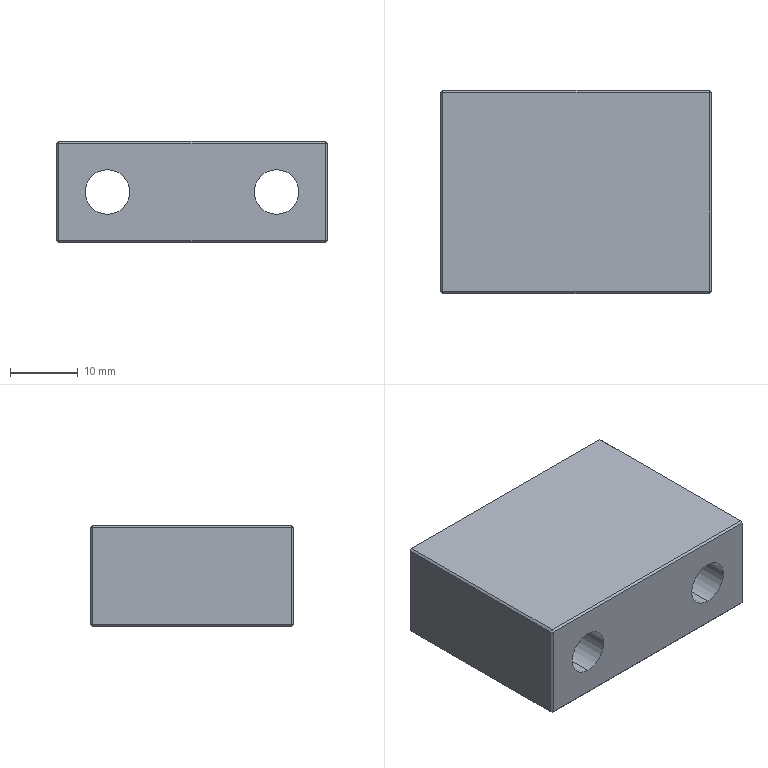Part | SolidWorks | features Chamfer 1, Extrusion 1, HoleWzd 1 | 1 solid | 36 faces | box 40 x 30 x 15 mm | volume 15105 mm3 | plane 28 | cylinder 8 | commonest cylinder face diameters 6.6 x4 11 x4
STEP:
#1=CARTESIAN_POINT('',(-12.5,8.2,2.));
#2=VERTEX_POINT('',#1);
#3=CARTESIAN_POINT('',(-12.5,8.2,13.));
#4=VERTEX_POINT('',#3);
#5=CARTESIAN_POINT('',(-12.5,8.2,7.5));
#6=DIRECTION('',(0.,1.,0.));
#7=DIRECTION('',(0.,0.,1.));
#8=AXIS2_PLACEMENT_3D('',#5,#6,#7);
#9=CIRCLE('',#8,5.5);
#10=EDGE_CURVE('',#2,#4,#9,.T.);
#11=ORIENTED_EDGE('',*,*,#10,.F.);
#12=CARTESIAN_POINT('',(-12.5,15.,2.));
#13=VERTEX_POINT('',#12);
#14=CARTESIAN_POINT('',(-12.5,15.,2.));
#15=DIRECTION('',(0.,1.,0.));
#16=VECTOR('',#15,1000.);
#17=LINE('',#14,#16);
#18=EDGE_CURVE('',#2,#13,#17,.T.);
#19=ORIENTED_EDGE('',*,*,#18,.T.);
#20=CARTESIAN_POINT('',(-12.5,15.,13.));
#21=VERTEX_POINT('',#20);
#22=CARTESIAN_POINT('',(-12.5,15.,7.5));
#23=DIRECTION('',(0.,1.,0.));
#24=DIRECTION('',(0.,0.,1.));
#25=AXIS2_PLACEMENT_3D('',#22,#23,#24);
#26=CIRCLE('',#25,5.5);
#27=EDGE_CURVE('',#13,#21,#26,.T.);
#28=ORIENTED_EDGE('',*,*,#27,.T.);
#29=CARTESIAN_POINT('',(-12.5,15.,13.));
#30=DIRECTION('',(0.,1.,0.));
#31=VECTOR('',#30,1000.);
#32=LINE('',#29,#31);
#33=EDGE_CURVE('',#4,#21,#32,.T.);
#34=ORIENTED_EDGE('',*,*,#33,.F.);
#35=EDGE_LOOP('',(#11,#19,#28,#34));
#36=FACE_OUTER_BOUND('',#35,.T.);
#37=CARTESIAN_POINT('',(-12.5,15.,7.5));
#38=DIRECTION('',(0.,1.,0.));
#39=DIRECTION('',(0.,0.,1.));
#40=AXIS2_PLACEMENT_3D('',#37,#38,#39);
#41=CYLINDRICAL_SURFACE('',#40,5.5);
#42=ADVANCED_FACE('',(#36),#41,.F.);
#43=CARTESIAN_POINT('',(-12.5,-15.,4.2));
#44=VERTEX_POINT('',#43);
#45=CARTESIAN_POINT('',(-12.5,-15.,10.8));
#46=VERTEX_POINT('',#45);
#47=CARTESIAN_POINT('',(-12.5,-15.,7.5));
#48=DIRECTION('',(0.,1.,0.));
#49=DIRECTION('',(0.,0.,1.));
#50=AXIS2_PLACEMENT_3D('',#47,#48,#49);
#51=CIRCLE('',#50,3.3);
#52=EDGE_CURVE('',#44,#46,#51,.T.);
#53=ORIENTED_EDGE('',*,*,#52,.F.);
#54=CARTESIAN_POINT('',(-12.5,8.2,4.2));
#55=VERTEX_POINT('',#54);
#56=CARTESIAN_POINT('',(-12.5,15.,4.2));
#57=DIRECTION('',(0.,1.,0.));
#58=VECTOR('',#57,1000.);
#59=LINE('',#56,#58);
#60=EDGE_CURVE('',#44,#55,#59,.T.);
#61=ORIENTED_EDGE('',*,*,#60,.T.);
#62=CARTESIAN_POINT('',(-12.5,8.2,10.8));
#63=VERTEX_POINT('',#62);
#64=CARTESIAN_POINT('',(-12.5,8.2,7.5));
#65=DIRECTION('',(0.,1.,0.));
#66=DIRECTION('',(0.,0.,1.));
#67=AXIS2_PLACEMENT_3D('',#64,#65,#66);
#68=CIRCLE('',#67,3.3);
#69=EDGE_CURVE('',#55,#63,#68,.T.);
#70=ORIENTED_EDGE('',*,*,#69,.T.);
#71=CARTESIAN_POINT('',(-12.5,15.,10.8));
#72=DIRECTION('',(0.,1.,0.));
#73=VECTOR('',#72,1000.);
#74=LINE('',#71,#73);
#75=EDGE_CURVE('',#46,#63,#74,.T.);
#76=ORIENTED_EDGE('',*,*,#75,.F.);
#77=EDGE_LOOP('',(#53,#61,#70,#76));
#78=FACE_OUTER_BOUND('',#77,.T.);
#79=CARTESIAN_POINT('',(-12.5,15.,7.5));
#80=DIRECTION('',(0.,1.,0.));
#81=DIRECTION('',(0.,0.,1.));
#82=AXIS2_PLACEMENT_3D('',#79,#80,#81);
#83=CYLINDRICAL_SURFACE('',#82,3.3);
#84=ADVANCED_FACE('',(#78),#83,.F.);
#85=CARTESIAN_POINT('',(12.5,8.2,2.));
#86=VERTEX_POINT('',#85);
#87=CARTESIAN_POINT('',(12.5,8.2,13.));
#88=VERTEX_POINT('',#87);
#89=CARTESIAN_POINT('',(12.5,8.2,7.5));
#90=DIRECTION('',(0.,1.,0.));
#91=DIRECTION('',(0.,0.,1.));
#92=AXIS2_PLACEMENT_3D('',#89,#90,#91);
#93=CIRCLE('',#92,5.5);
#94=EDGE_CURVE('',#86,#88,#93,.T.);
#95=ORIENTED_EDGE('',*,*,#94,.F.);
#96=CARTESIAN_POINT('',(12.5,15.,2.));
#97=VERTEX_POINT('',#96);
#98=CARTESIAN_POINT('',(12.5,15.,2.));
#99=DIRECTION('',(0.,1.,0.));
#100=VECTOR('',#99,1000.);
#101=LINE('',#98,#100);
#102=EDGE_CURVE('',#86,#97,#101,.T.);
#103=ORIENTED_EDGE('',*,*,#102,.T.);
#104=CARTESIAN_POINT('',(12.5,15.,13.));
#105=VERTEX_POINT('',#104);
#106=CARTESIAN_POINT('',(12.5,15.,7.5));
#107=DIRECTION('',(0.,1.,0.));
#108=DIRECTION('',(0.,0.,1.));
#109=AXIS2_PLACEMENT_3D('',#106,#107,#108);
#110=CIRCLE('',#109,5.5);
#111=EDGE_CURVE('',#97,#105,#110,.T.);
#112=ORIENTED_EDGE('',*,*,#111,.T.);
#113=CARTESIAN_POINT('',(12.5,15.,13.));
#114=DIRECTION('',(0.,1.,0.));
#115=VECTOR('',#114,1000.);
#116=LINE('',#113,#115);
#117=EDGE_CURVE('',#88,#105,#116,.T.);
#118=ORIENTED_EDGE('',*,*,#117,.F.);
#119=EDGE_LOOP('',(#95,#103,#112,#118));
#120=FACE_OUTER_BOUND('',#119,.T.);
#121=CARTESIAN_POINT('',(12.5,15.,7.5));
#122=DIRECTION('',(0.,1.,0.));
#123=DIRECTION('',(0.,0.,1.));
#124=AXIS2_PLACEMENT_3D('',#121,#122,#123);
#125=CYLINDRICAL_SURFACE('',#124,5.5);
#126=ADVANCED_FACE('',(#120),#125,.F.);
#127=CARTESIAN_POINT('',(12.5,-15.,4.2));
#128=VERTEX_POINT('',#127);
#129=CARTESIAN_POINT('',(12.5,-15.,10.8));
#130=VERTEX_POINT('',#129);
#131=CARTESIAN_POINT('',(12.5,-15.,7.5));
#132=DIRECTION('',(0.,1.,0.));
#133=DIRECTION('',(0.,0.,1.));
#134=AXIS2_PLACEMENT_3D('',#131,#132,#133);
#135=CIRCLE('',#134,3.3);
#136=EDGE_CURVE('',#128,#130,#135,.T.);
#137=ORIENTED_EDGE('',*,*,#136,.F.);
#138=CARTESIAN_POINT('',(12.5,8.2,4.2));
#139=VERTEX_POINT('',#138);
#140=CARTESIAN_POINT('',(12.5,15.,4.2));
#141=DIRECTION('',(0.,1.,0.));
#142=VECTOR('',#141,1000.);
#143=LINE('',#140,#142);
#144=EDGE_CURVE('',#128,#139,#143,.T.);
#145=ORIENTED_EDGE('',*,*,#144,.T.);
#146=CARTESIAN_POINT('',(12.5,8.2,10.8));
#147=VERTEX_POINT('',#146);
#148=CARTESIAN_POINT('',(12.5,8.2,7.5));
#149=DIRECTION('',(0.,1.,0.));
#150=DIRECTION('',(0.,0.,1.));
#151=AXIS2_PLACEMENT_3D('',#148,#149,#150);
#152=CIRCLE('',#151,3.3);
#153=EDGE_CURVE('',#139,#147,#152,.T.);
#154=ORIENTED_EDGE('',*,*,#153,.T.);
#155=CARTESIAN_POINT('',(12.5,15.,10.8));
#156=DIRECTION('',(0.,1.,0.));
#157=VECTOR('',#156,1000.);
#158=LINE('',#155,#157);
#159=EDGE_CURVE('',#130,#147,#158,.T.);
#160=ORIENTED_EDGE('',*,*,#159,.F.);
#161=EDGE_LOOP('',(#137,#145,#154,#160));
#162=FACE_OUTER_BOUND('',#161,.T.);
#163=CARTESIAN_POINT('',(12.5,15.,7.5));
#164=DIRECTION('',(0.,1.,0.));
#165=DIRECTION('',(0.,0.,1.));
#166=AXIS2_PLACEMENT_3D('',#163,#164,#165);
#167=CYLINDRICAL_SURFACE('',#166,3.3);
#168=ADVANCED_FACE('',(#162),#167,.F.);
#169=CARTESIAN_POINT('',(20.,14.7,14.7));
#170=VERTEX_POINT('',#169);
#171=CARTESIAN_POINT('',(20.,-14.7,14.7));
#172=VERTEX_POINT('',#171);
#173=CARTESIAN_POINT('',(20.,-15.,14.7));
#174=DIRECTION('',(0.,-1.,0.));
#175=VECTOR('',#174,1000.);
#176=LINE('',#173,#175);
#177=EDGE_CURVE('',#170,#172,#176,.T.);
#178=ORIENTED_EDGE('',*,*,#177,.T.);
#179=CARTESIAN_POINT('',(20.,-14.7,0.3));
#180=VERTEX_POINT('',#179);
#181=CARTESIAN_POINT('',(20.,-14.7,15.));
#182=DIRECTION('',(0.,0.,-1.));
#183=VECTOR('',#182,1000.);
#184=LINE('',#181,#183);
#185=EDGE_CURVE('',#172,#180,#184,.T.);
#186=ORIENTED_EDGE('',*,*,#185,.T.);
#187=CARTESIAN_POINT('',(20.,14.7,0.3));
#188=VERTEX_POINT('',#187);
#189=CARTESIAN_POINT('',(20.,15.,0.3));
#190=DIRECTION('',(0.,1.,0.));
#191=VECTOR('',#190,1000.);
#192=LINE('',#189,#191);
#193=EDGE_CURVE('',#180,#188,#192,.T.);
#194=ORIENTED_EDGE('',*,*,#193,.T.);
#195=CARTESIAN_POINT('',(20.,14.7,15.));
#196=DIRECTION('',(0.,0.,1.));
#197=VECTOR('',#196,1000.);
#198=LINE('',#195,#197);
#199=EDGE_CURVE('',#188,#170,#198,.T.);
#200=ORIENTED_EDGE('',*,*,#199,.T.);
#201=EDGE_LOOP('',(#178,#186,#194,#200));
#202=FACE_OUTER_BOUND('',#201,.T.);
#203=CARTESIAN_POINT('',(20.,15.,15.));
#204=DIRECTION('',(-1.,0.,0.));
#205=DIRECTION('',(0.,-1.,0.));
#206=AXIS2_PLACEMENT_3D('',#203,#204,#205);
#207=PLANE('',#206);
#208=ADVANCED_FACE('',(#202),#207,.F.);
#209=CARTESIAN_POINT('',(19.7,15.,0.3));
#210=VERTEX_POINT('',#209);
#211=CARTESIAN_POINT('',(-19.7,15.,0.3));
#212=VERTEX_POINT('',#211);
#213=CARTESIAN_POINT('',(-20.,15.,0.3));
#214=DIRECTION('',(-1.,0.,0.));
#215=VECTOR('',#214,1000.);
#216=LINE('',#213,#215);
#217=EDGE_CURVE('',#210,#212,#216,.T.);
#218=ORIENTED_EDGE('',*,*,#217,.T.);
#219=CARTESIAN_POINT('',(-19.7,15.,14.7));
#220=VERTEX_POINT('',#219);
#221=CARTESIAN_POINT('',(-19.7,15.,15.));
#222=DIRECTION('',(0.,0.,1.));
#223=VECTOR('',#222,1000.);
#224=LINE('',#221,#223);
#225=EDGE_CURVE('',#212,#220,#224,.T.);
#226=ORIENTED_EDGE('',*,*,#225,.T.);
#227=CARTESIAN_POINT('',(19.7,15.,14.7));
#228=VERTEX_POINT('',#227);
#229=CARTESIAN_POINT('',(20.,15.,14.7));
#230=DIRECTION('',(1.,0.,0.));
#231=VECTOR('',#230,1000.);
#232=LINE('',#229,#231);
#233=EDGE_CURVE('',#220,#228,#232,.T.);
#234=ORIENTED_EDGE('',*,*,#233,.T.);
#235=CARTESIAN_POINT('',(19.7,15.,15.));
#236=DIRECTION('',(0.,0.,-1.));
#237=VECTOR('',#236,1000.);
#238=LINE('',#235,#237);
#239=EDGE_CURVE('',#228,#210,#238,.T.);
#240=ORIENTED_EDGE('',*,*,#239,.T.);
#241=EDGE_LOOP('',(#218,#226,#234,#240));
#242=FACE_OUTER_BOUND('',#241,.T.);
#243=CARTESIAN_POINT('',(-12.5,15.,7.5));
#244=DIRECTION('',(0.,1.,0.));
#245=DIRECTION('',(0.,0.,1.));
#246=AXIS2_PLACEMENT_3D('',#243,#244,#245);
#247=CIRCLE('',#246,5.5);
#248=EDGE_CURVE('',#21,#13,#247,.T.);
#249=ORIENTED_EDGE('',*,*,#248,.F.);
#250=ORIENTED_EDGE('',*,*,#27,.F.);
#251=EDGE_LOOP('',(#249,#250));
#252=FACE_BOUND('',#251,.T.);
#253=CARTESIAN_POINT('',(12.5,15.,7.5));
#254=DIRECTION('',(0.,1.,0.));
#255=DIRECTION('',(0.,0.,1.));
#256=AXIS2_PLACEMENT_3D('',#253,#254,#255);
#257=CIRCLE('',#256,5.5);
#258=EDGE_CURVE('',#105,#97,#257,.T.);
#259=ORIENTED_EDGE('',*,*,#258,.F.);
#260=ORIENTED_EDGE('',*,*,#111,.F.);
#261=EDGE_LOOP('',(#259,#260));
#262=FACE_BOUND('',#261,.T.);
#263=CARTESIAN_POINT('',(-20.,15.,15.));
#264=DIRECTION('',(0.,-1.,0.));
#265=DIRECTION('',(0.,0.,-1.));
#266=AXIS2_PLACEMENT_3D('',#263,#264,#265);
#267=PLANE('',#266);
#268=ADVANCED_FACE('',(#242,#252,#262),#267,.F.);
#269=CARTESIAN_POINT('',(-20.,-14.7,0.3));
#270=VERTEX_POINT('',#269);
#271=CARTESIAN_POINT('',(-20.,-14.7,14.7));
#272=VERTEX_POINT('',#271);
#273=CARTESIAN_POINT('',(-20.,-14.7,15.));
#274=DIRECTION('',(0.,0.,1.));
#275=VECTOR('',#274,1000.);
#276=LINE('',#273,#275);
#277=EDGE_CURVE('',#270,#272,#276,.T.);
#278=ORIENTED_EDGE('',*,*,#277,.T.);
#279=CARTESIAN_POINT('',(-20.,14.7,14.7));
#280=VERTEX_POINT('',#279);
#281=CARTESIAN_POINT('',(-20.,15.,14.7));
#282=DIRECTION('',(0.,1.,0.));
#283=VECTOR('',#282,1000.);
#284=LINE('',#281,#283);
#285=EDGE_CURVE('',#272,#280,#284,.T.);
#286=ORIENTED_EDGE('',*,*,#285,.T.);
#287=CARTESIAN_POINT('',(-20.,14.7,0.3));
#288=VERTEX_POINT('',#287);
#289=CARTESIAN_POINT('',(-20.,14.7,15.));
#290=DIRECTION('',(0.,0.,-1.));
#291=VECTOR('',#290,1000.);
#292=LINE('',#289,#291);
#293=EDGE_CURVE('',#280,#288,#292,.T.);
#294=ORIENTED_EDGE('',*,*,#293,.T.);
#295=CARTESIAN_POINT('',(-20.,15.,0.3));
#296=DIRECTION('',(0.,-1.,0.));
#297=VECTOR('',#296,1000.);
#298=LINE('',#295,#297);
#299=EDGE_CURVE('',#288,#270,#298,.T.);
#300=ORIENTED_EDGE('',*,*,#299,.T.);
#301=EDGE_LOOP('',(#278,#286,#294,#300));
#302=FACE_OUTER_BOUND('',#301,.T.);
#303=CARTESIAN_POINT('',(-20.,15.,15.));
#304=DIRECTION('',(1.,0.,0.));
#305=DIRECTION('',(0.,1.,0.));
#306=AXIS2_PLACEMENT_3D('',#303,#304,#305);
#307=PLANE('',#306);
#308=ADVANCED_FACE('',(#302),#307,.F.);
#309=CARTESIAN_POINT('',(19.7,-15.,0.3));
#310=VERTEX_POINT('',#309);
#311=CARTESIAN_POINT('',(19.7,-15.,14.7));
#312=VERTEX_POINT('',#311);
#313=CARTESIAN_POINT('',(19.7,-15.,15.));
#314=DIRECTION('',(0.,0.,1.));
#315=VECTOR('',#314,1000.);
#316=LINE('',#313,#315);
#317=EDGE_CURVE('',#310,#312,#316,.T.);
#318=ORIENTED_EDGE('',*,*,#317,.T.);
#319=CARTESIAN_POINT('',(-19.7,-15.,14.7));
#320=VERTEX_POINT('',#319);
#321=CARTESIAN_POINT('',(-20.,-15.,14.7));
#322=DIRECTION('',(-1.,0.,0.));
#323=VECTOR('',#322,1000.);
#324=LINE('',#321,#323);
#325=EDGE_CURVE('',#312,#320,#324,.T.);
#326=ORIENTED_EDGE('',*,*,#325,.T.);
#327=CARTESIAN_POINT('',(-19.7,-15.,0.3));
#328=VERTEX_POINT('',#327);
#329=CARTESIAN_POINT('',(-19.7,-15.,15.));
#330=DIRECTION('',(0.,0.,-1.));
#331=VECTOR('',#330,1000.);
#332=LINE('',#329,#331);
#333=EDGE_CURVE('',#320,#328,#332,.T.);
#334=ORIENTED_EDGE('',*,*,#333,.T.);
#335=CARTESIAN_POINT('',(-20.,-15.,0.3));
#336=DIRECTION('',(1.,0.,0.));
#337=VECTOR('',#336,1000.);
#338=LINE('',#335,#337);
#339=EDGE_CURVE('',#328,#310,#338,.T.);
#340=ORIENTED_EDGE('',*,*,#339,.T.);
#341=EDGE_LOOP('',(#318,#326,#334,#340));
#342=FACE_OUTER_BOUND('',#341,.T.);
#343=CARTESIAN_POINT('',(-12.5,-15.,7.5));
#344=DIRECTION('',(0.,1.,0.));
#345=DIRECTION('',(0.,0.,1.));
#346=AXIS2_PLACEMENT_3D('',#343,#344,#345);
#347=CIRCLE('',#346,3.3);
#348=EDGE_CURVE('',#46,#44,#347,.T.);
#349=ORIENTED_EDGE('',*,*,#348,.T.);
#350=ORIENTED_EDGE('',*,*,#52,.T.);
#351=EDGE_LOOP('',(#349,#350));
#352=FACE_BOUND('',#351,.T.);
#353=CARTESIAN_POINT('',(12.5,-15.,7.5));
#354=DIRECTION('',(0.,1.,0.));
#355=DIRECTION('',(0.,0.,1.));
#356=AXIS2_PLACEMENT_3D('',#353,#354,#355);
#357=CIRCLE('',#356,3.3);
#358=EDGE_CURVE('',#130,#128,#357,.T.);
#359=ORIENTED_EDGE('',*,*,#358,.T.);
#360=ORIENTED_EDGE('',*,*,#136,.T.);
#361=EDGE_LOOP('',(#359,#360));
#362=FACE_BOUND('',#361,.T.);
#363=CARTESIAN_POINT('',(-20.,-15.,15.));
#364=DIRECTION('',(0.,1.,0.));
#365=DIRECTION('',(0.,0.,1.));
#366=AXIS2_PLACEMENT_3D('',#363,#364,#365);
#367=PLANE('',#366);
#368=ADVANCED_FACE('',(#342,#352,#362),#367,.F.);
#369=CARTESIAN_POINT('',(-19.7,14.7,15.));
#370=VERTEX_POINT('',#369);
#371=CARTESIAN_POINT('',(-19.7,-14.7,15.));
#372=VERTEX_POINT('',#371);
#373=CARTESIAN_POINT('',(-19.7,-15.,15.));
#374=DIRECTION('',(0.,-1.,0.));
#375=VECTOR('',#374,1000.);
#376=LINE('',#373,#375);
#377=EDGE_CURVE('',#370,#372,#376,.T.);
#378=ORIENTED_EDGE('',*,*,#377,.T.);
#379=CARTESIAN_POINT('',(19.7,-14.7,15.));
#380=VERTEX_POINT('',#379);
#381=CARTESIAN_POINT('',(20.,-14.7,15.));
#382=DIRECTION('',(1.,0.,0.));
#383=VECTOR('',#382,1000.);
#384=LINE('',#381,#383);
#385=EDGE_CURVE('',#372,#380,#384,.T.);
#386=ORIENTED_EDGE('',*,*,#385,.T.);
#387=CARTESIAN_POINT('',(19.7,14.7,15.));
#388=VERTEX_POINT('',#387);
#389=CARTESIAN_POINT('',(19.7,15.,15.));
#390=DIRECTION('',(0.,1.,0.));
#391=VECTOR('',#390,1000.);
#392=LINE('',#389,#391);
#393=EDGE_CURVE('',#380,#388,#392,.T.);
#394=ORIENTED_EDGE('',*,*,#393,.T.);
#395=CARTESIAN_POINT('',(-20.,14.7,15.));
#396=DIRECTION('',(-1.,0.,0.));
#397=VECTOR('',#396,1000.);
#398=LINE('',#395,#397);
#399=EDGE_CURVE('',#388,#370,#398,.T.);
#400=ORIENTED_EDGE('',*,*,#399,.T.);
#401=EDGE_LOOP('',(#378,#386,#394,#400));
#402=FACE_OUTER_BOUND('',#401,.T.);
#403=CARTESIAN_POINT('',(0.,0.,15.));
#404=DIRECTION('',(0.,0.,1.));
#405=DIRECTION('',(1.,0.,0.));
#406=AXIS2_PLACEMENT_3D('',#403,#404,#405);
#407=PLANE('',#406);
#408=ADVANCED_FACE('',(#402),#407,.T.);
#409=CARTESIAN_POINT('',(-19.7,-14.7,0.));
#410=VERTEX_POINT('',#409);
#411=CARTESIAN_POINT('',(-19.7,14.7,0.));
#412=VERTEX_POINT('',#411);
#413=CARTESIAN_POINT('',(-19.7,0.,0.));
#414=DIRECTION('',(0.,1.,0.));
#415=VECTOR('',#414,1000.);
#416=LINE('',#413,#415);
#417=EDGE_CURVE('',#410,#412,#416,.T.);
#418=ORIENTED_EDGE('',*,*,#417,.T.);
#419=CARTESIAN_POINT('',(19.7,14.7,0.));
#420=VERTEX_POINT('',#419);
#421=CARTESIAN_POINT('',(0.,14.7,0.));
#422=DIRECTION('',(1.,0.,0.));
#423=VECTOR('',#422,1000.);
#424=LINE('',#421,#423);
#425=EDGE_CURVE('',#412,#420,#424,.T.);
#426=ORIENTED_EDGE('',*,*,#425,.T.);
#427=CARTESIAN_POINT('',(19.7,-14.7,0.));
#428=VERTEX_POINT('',#427);
#429=CARTESIAN_POINT('',(19.7,0.,0.));
#430=DIRECTION('',(0.,-1.,0.));
#431=VECTOR('',#430,1000.);
#432=LINE('',#429,#431);
#433=EDGE_CURVE('',#420,#428,#432,.T.);
#434=ORIENTED_EDGE('',*,*,#433,.T.);
#435=CARTESIAN_POINT('',(0.,-14.7,0.));
#436=DIRECTION('',(-1.,0.,0.));
#437=VECTOR('',#436,1000.);
#438=LINE('',#435,#437);
#439=EDGE_CURVE('',#428,#410,#438,.T.);
#440=ORIENTED_EDGE('',*,*,#439,.T.);
#441=EDGE_LOOP('',(#418,#426,#434,#440));
#442=FACE_OUTER_BOUND('',#441,.T.);
#443=CARTESIAN_POINT('',(0.,0.,0.));
#444=DIRECTION('',(0.,0.,1.));
#445=DIRECTION('',(1.,0.,0.));
#446=AXIS2_PLACEMENT_3D('',#443,#444,#445);
#447=PLANE('',#446);
#448=ADVANCED_FACE('',(#442),#447,.F.);
#449=ORIENTED_EDGE('',*,*,#144,.F.);
#450=ORIENTED_EDGE('',*,*,#358,.F.);
#451=ORIENTED_EDGE('',*,*,#159,.T.);
#452=CARTESIAN_POINT('',(12.5,8.2,7.5));
#453=DIRECTION('',(0.,1.,0.));
#454=DIRECTION('',(0.,0.,1.));
#455=AXIS2_PLACEMENT_3D('',#452,#453,#454);
#456=CIRCLE('',#455,3.3);
#457=EDGE_CURVE('',#147,#139,#456,.T.);
#458=ORIENTED_EDGE('',*,*,#457,.T.);
#459=EDGE_LOOP('',(#449,#450,#451,#458));
#460=FACE_OUTER_BOUND('',#459,.T.);
#461=CARTESIAN_POINT('',(12.5,15.,7.5));
#462=DIRECTION('',(0.,1.,0.));
#463=DIRECTION('',(0.,0.,1.));
#464=AXIS2_PLACEMENT_3D('',#461,#462,#463);
#465=CYLINDRICAL_SURFACE('',#464,3.3);
#466=ADVANCED_FACE('',(#460),#465,.F.);
#467=ORIENTED_EDGE('',*,*,#457,.F.);
#468=ORIENTED_EDGE('',*,*,#153,.F.);
#469=EDGE_LOOP('',(#467,#468));
#470=FACE_BOUND('',#469,.T.);
#471=CARTESIAN_POINT('',(12.5,8.2,7.5));
#472=DIRECTION('',(0.,1.,0.));
#473=DIRECTION('',(0.,0.,1.));
#474=AXIS2_PLACEMENT_3D('',#471,#472,#473);
#475=CIRCLE('',#474,5.5);
#476=EDGE_CURVE('',#88,#86,#475,.T.);
#477=ORIENTED_EDGE('',*,*,#476,.T.);
#478=ORIENTED_EDGE('',*,*,#94,.T.);
#479=EDGE_LOOP('',(#477,#478));
#480=FACE_OUTER_BOUND('',#479,.T.);
#481=CARTESIAN_POINT('',(15.8,8.2,7.5));
#482=DIRECTION('',(0.,-1.,0.));
#483=DIRECTION('',(0.,0.,-1.));
#484=AXIS2_PLACEMENT_3D('',#481,#482,#483);
#485=PLANE('',#484);
#486=ADVANCED_FACE('',(#470,#480),#485,.F.);
#487=ORIENTED_EDGE('',*,*,#102,.F.);
#488=ORIENTED_EDGE('',*,*,#476,.F.);
#489=ORIENTED_EDGE('',*,*,#117,.T.);
#490=ORIENTED_EDGE('',*,*,#258,.T.);
#491=EDGE_LOOP('',(#487,#488,#489,#490));
#492=FACE_OUTER_BOUND('',#491,.T.);
#493=CARTESIAN_POINT('',(12.5,15.,7.5));
#494=DIRECTION('',(0.,1.,0.));
#495=DIRECTION('',(0.,0.,1.));
#496=AXIS2_PLACEMENT_3D('',#493,#494,#495);
#497=CYLINDRICAL_SURFACE('',#496,5.5);
#498=ADVANCED_FACE('',(#492),#497,.F.);
#499=ORIENTED_EDGE('',*,*,#60,.F.);
#500=ORIENTED_EDGE('',*,*,#348,.F.);
#501=ORIENTED_EDGE('',*,*,#75,.T.);
#502=CARTESIAN_POINT('',(-12.5,8.2,7.5));
#503=DIRECTION('',(0.,1.,0.));
#504=DIRECTION('',(0.,0.,1.));
#505=AXIS2_PLACEMENT_3D('',#502,#503,#504);
#506=CIRCLE('',#505,3.3);
#507=EDGE_CURVE('',#63,#55,#506,.T.);
#508=ORIENTED_EDGE('',*,*,#507,.T.);
#509=EDGE_LOOP('',(#499,#500,#501,#508));
#510=FACE_OUTER_BOUND('',#509,.T.);
#511=CARTESIAN_POINT('',(-12.5,15.,7.5));
#512=DIRECTION('',(0.,1.,0.));
#513=DIRECTION('',(0.,0.,1.));
#514=AXIS2_PLACEMENT_3D('',#511,#512,#513);
#515=CYLINDRICAL_SURFACE('',#514,3.3);
#516=ADVANCED_FACE('',(#510),#515,.F.);
#517=ORIENTED_EDGE('',*,*,#507,.F.);
#518=ORIENTED_EDGE('',*,*,#69,.F.);
#519=EDGE_LOOP('',(#517,#518));
#520=FACE_BOUND('',#519,.T.);
#521=CARTESIAN_POINT('',(-12.5,8.2,7.5));
#522=DIRECTION('',(0.,1.,0.));
#523=DIRECTION('',(0.,0.,1.));
#524=AXIS2_PLACEMENT_3D('',#521,#522,#523);
#525=CIRCLE('',#524,5.5);
#526=EDGE_CURVE('',#4,#2,#525,.T.);
#527=ORIENTED_EDGE('',*,*,#526,.T.);
#528=ORIENTED_EDGE('',*,*,#10,.T.);
#529=EDGE_LOOP('',(#527,#528));
#530=FACE_OUTER_BOUND('',#529,.T.);
#531=CARTESIAN_POINT('',(-9.2,8.2,7.5));
#532=DIRECTION('',(0.,-1.,0.));
#533=DIRECTION('',(0.,0.,-1.));
#534=AXIS2_PLACEMENT_3D('',#531,#532,#533);
#535=PLANE('',#534);
#536=ADVANCED_FACE('',(#520,#530),#535,.F.);
#537=ORIENTED_EDGE('',*,*,#18,.F.);
#538=ORIENTED_EDGE('',*,*,#526,.F.);
#539=ORIENTED_EDGE('',*,*,#33,.T.);
#540=ORIENTED_EDGE('',*,*,#248,.T.);
#541=EDGE_LOOP('',(#537,#538,#539,#540));
#542=FACE_OUTER_BOUND('',#541,.T.);
#543=CARTESIAN_POINT('',(-12.5,15.,7.5));
#544=DIRECTION('',(0.,1.,0.));
#545=DIRECTION('',(0.,0.,1.));
#546=AXIS2_PLACEMENT_3D('',#543,#544,#545);
#547=CYLINDRICAL_SURFACE('',#546,5.5);
#548=ADVANCED_FACE('',(#542),#547,.F.);
#549=CARTESIAN_POINT('',(19.7,-15.,14.7));
#550=DIRECTION('',(0.7071,0.7071,0.));
#551=VECTOR('',#550,1000.);
#552=LINE('',#549,#551);
#553=EDGE_CURVE('',#312,#172,#552,.T.);
#554=ORIENTED_EDGE('',*,*,#553,.F.);
#555=ORIENTED_EDGE('',*,*,#317,.F.);
#556=CARTESIAN_POINT('',(20.,-14.7,0.3));
#557=DIRECTION('',(-0.7071,-0.7071,0.));
#558=VECTOR('',#557,1000.);
#559=LINE('',#556,#558);
#560=EDGE_CURVE('',#180,#310,#559,.T.);
#561=ORIENTED_EDGE('',*,*,#560,.F.);
#562=ORIENTED_EDGE('',*,*,#185,.F.);
#563=EDGE_LOOP('',(#554,#555,#561,#562));
#564=FACE_OUTER_BOUND('',#563,.T.);
#565=CARTESIAN_POINT('',(20.,-14.7,15.));
#566=DIRECTION('',(-0.7071,0.7071,0.));
#567=DIRECTION('',(0.,0.,-1.));
#568=AXIS2_PLACEMENT_3D('',#565,#566,#567);
#569=PLANE('',#568);
#570=ADVANCED_FACE('',(#564),#569,.F.);
#571=CARTESIAN_POINT('',(19.7,-15.,14.7));
#572=DIRECTION('',(0.,0.7071,0.7071));
#573=VECTOR('',#572,1000.);
#574=LINE('',#571,#573);
#575=EDGE_CURVE('',#312,#380,#574,.T.);
#576=ORIENTED_EDGE('',*,*,#575,.F.);
#577=ORIENTED_EDGE('',*,*,#553,.T.);
#578=CARTESIAN_POINT('',(19.85,-14.7,14.85));
#579=DIRECTION('',(0.7071,0.,-0.7071));
#580=VECTOR('',#579,1000.);
#581=LINE('',#578,#580);
#582=EDGE_CURVE('',#380,#172,#581,.T.);
#583=ORIENTED_EDGE('',*,*,#582,.F.);
#584=EDGE_LOOP('',(#576,#577,#583));
#585=FACE_OUTER_BOUND('',#584,.T.);
#586=CARTESIAN_POINT('',(19.7,-15.,14.7));
#587=DIRECTION('',(0.5774,-0.5774,0.5774));
#588=DIRECTION('',(0.7071,0.,-0.7071));
#589=AXIS2_PLACEMENT_3D('',#586,#587,#588);
#590=PLANE('',#589);
#591=ADVANCED_FACE('',(#585),#590,.T.);
#592=CARTESIAN_POINT('',(20.,-14.7,0.3));
#593=DIRECTION('',(-0.7071,0.,-0.7071));
#594=VECTOR('',#593,1000.);
#595=LINE('',#592,#594);
#596=EDGE_CURVE('',#180,#428,#595,.T.);
#597=ORIENTED_EDGE('',*,*,#596,.F.);
#598=ORIENTED_EDGE('',*,*,#560,.T.);
#599=CARTESIAN_POINT('',(19.7,-14.85,0.15));
#600=DIRECTION('',(0.,-0.7071,0.7071));
#601=VECTOR('',#600,1000.);
#602=LINE('',#599,#601);
#603=EDGE_CURVE('',#428,#310,#602,.T.);
#604=ORIENTED_EDGE('',*,*,#603,.F.);
#605=EDGE_LOOP('',(#597,#598,#604));
#606=FACE_OUTER_BOUND('',#605,.T.);
#607=CARTESIAN_POINT('',(20.,-14.7,0.3));
#608=DIRECTION('',(0.5774,-0.5774,-0.5774));
#609=DIRECTION('',(-0.7071,0.,-0.7071));
#610=AXIS2_PLACEMENT_3D('',#607,#608,#609);
#611=PLANE('',#610);
#612=ADVANCED_FACE('',(#606),#611,.T.);
#613=ORIENTED_EDGE('',*,*,#582,.T.);
#614=ORIENTED_EDGE('',*,*,#177,.F.);
#615=CARTESIAN_POINT('',(19.85,14.7,14.85));
#616=DIRECTION('',(0.7071,0.,-0.7071));
#617=VECTOR('',#616,1000.);
#618=LINE('',#615,#617);
#619=EDGE_CURVE('',#388,#170,#618,.T.);
#620=ORIENTED_EDGE('',*,*,#619,.F.);
#621=ORIENTED_EDGE('',*,*,#393,.F.);
#622=EDGE_LOOP('',(#613,#614,#620,#621));
#623=FACE_OUTER_BOUND('',#622,.T.);
#624=CARTESIAN_POINT('',(19.7,0.,15.));
#625=DIRECTION('',(0.7071,0.,0.7071));
#626=DIRECTION('',(0.,-1.,0.));
#627=AXIS2_PLACEMENT_3D('',#624,#625,#626);
#628=PLANE('',#627);
#629=ADVANCED_FACE('',(#623),#628,.T.);
#630=ORIENTED_EDGE('',*,*,#575,.T.);
#631=ORIENTED_EDGE('',*,*,#385,.F.);
#632=CARTESIAN_POINT('',(-19.7,-14.85,14.85));
#633=DIRECTION('',(0.,0.7071,0.7071));
#634=VECTOR('',#633,1000.);
#635=LINE('',#632,#634);
#636=EDGE_CURVE('',#320,#372,#635,.T.);
#637=ORIENTED_EDGE('',*,*,#636,.F.);
#638=ORIENTED_EDGE('',*,*,#325,.F.);
#639=EDGE_LOOP('',(#630,#631,#637,#638));
#640=FACE_OUTER_BOUND('',#639,.T.);
#641=CARTESIAN_POINT('',(0.,-14.7,15.));
#642=DIRECTION('',(0.,-0.7071,0.7071));
#643=DIRECTION('',(-1.,0.,0.));
#644=AXIS2_PLACEMENT_3D('',#641,#642,#643);
#645=PLANE('',#644);
#646=ADVANCED_FACE('',(#640),#645,.T.);
#647=CARTESIAN_POINT('',(-19.7,-15.,0.3));
#648=DIRECTION('',(-0.7071,0.7071,0.));
#649=VECTOR('',#648,1000.);
#650=LINE('',#647,#649);
#651=EDGE_CURVE('',#328,#270,#650,.T.);
#652=ORIENTED_EDGE('',*,*,#651,.F.);
#653=ORIENTED_EDGE('',*,*,#333,.F.);
#654=CARTESIAN_POINT('',(-20.,-14.7,14.7));
#655=DIRECTION('',(0.7071,-0.7071,0.));
#656=VECTOR('',#655,1000.);
#657=LINE('',#654,#656);
#658=EDGE_CURVE('',#272,#320,#657,.T.);
#659=ORIENTED_EDGE('',*,*,#658,.F.);
#660=ORIENTED_EDGE('',*,*,#277,.F.);
#661=EDGE_LOOP('',(#652,#653,#659,#660));
#662=FACE_OUTER_BOUND('',#661,.T.);
#663=CARTESIAN_POINT('',(-19.7,-15.,15.));
#664=DIRECTION('',(0.7071,0.7071,0.));
#665=DIRECTION('',(0.,0.,-1.));
#666=AXIS2_PLACEMENT_3D('',#663,#664,#665);
#667=PLANE('',#666);
#668=ADVANCED_FACE('',(#662),#667,.F.);
#669=ORIENTED_EDGE('',*,*,#603,.T.);
#670=ORIENTED_EDGE('',*,*,#339,.F.);
#671=CARTESIAN_POINT('',(-19.7,-15.,0.3));
#672=DIRECTION('',(0.,-0.7071,0.7071));
#673=VECTOR('',#672,1000.);
#674=LINE('',#671,#673);
#675=EDGE_CURVE('',#410,#328,#674,.T.);
#676=ORIENTED_EDGE('',*,*,#675,.F.);
#677=ORIENTED_EDGE('',*,*,#439,.F.);
#678=EDGE_LOOP('',(#669,#670,#676,#677));
#679=FACE_OUTER_BOUND('',#678,.T.);
#680=CARTESIAN_POINT('',(-20.,-15.,0.3));
#681=DIRECTION('',(0.,0.7071,0.7071));
#682=DIRECTION('',(1.,0.,0.));
#683=AXIS2_PLACEMENT_3D('',#680,#681,#682);
#684=PLANE('',#683);
#685=ADVANCED_FACE('',(#679),#684,.F.);
#686=ORIENTED_EDGE('',*,*,#596,.T.);
#687=ORIENTED_EDGE('',*,*,#433,.F.);
#688=CARTESIAN_POINT('',(19.85,14.7,0.15));
#689=DIRECTION('',(-0.7071,0.,-0.7071));
#690=VECTOR('',#689,1000.);
#691=LINE('',#688,#690);
#692=EDGE_CURVE('',#188,#420,#691,.T.);
#693=ORIENTED_EDGE('',*,*,#692,.F.);
#694=ORIENTED_EDGE('',*,*,#193,.F.);
#695=EDGE_LOOP('',(#686,#687,#693,#694));
#696=FACE_OUTER_BOUND('',#695,.T.);
#697=CARTESIAN_POINT('',(20.,15.,0.3));
#698=DIRECTION('',(-0.7071,0.,0.7071));
#699=DIRECTION('',(0.,1.,0.));
#700=AXIS2_PLACEMENT_3D('',#697,#698,#699);
#701=PLANE('',#700);
#702=ADVANCED_FACE('',(#696),#701,.F.);
#703=CARTESIAN_POINT('',(19.7,15.,14.7));
#704=DIRECTION('',(-0.7071,0.7071,0.));
#705=VECTOR('',#704,1000.);
#706=LINE('',#703,#705);
#707=EDGE_CURVE('',#170,#228,#706,.T.);
#708=ORIENTED_EDGE('',*,*,#707,.F.);
#709=ORIENTED_EDGE('',*,*,#199,.F.);
#710=CARTESIAN_POINT('',(19.7,15.,0.3));
#711=DIRECTION('',(0.7071,-0.7071,0.));
#712=VECTOR('',#711,1000.);
#713=LINE('',#710,#712);
#714=EDGE_CURVE('',#210,#188,#713,.T.);
#715=ORIENTED_EDGE('',*,*,#714,.F.);
#716=ORIENTED_EDGE('',*,*,#239,.F.);
#717=EDGE_LOOP('',(#708,#709,#715,#716));
#718=FACE_OUTER_BOUND('',#717,.T.);
#719=CARTESIAN_POINT('',(19.7,15.,15.));
#720=DIRECTION('',(-0.7071,-0.7071,0.));
#721=DIRECTION('',(0.,0.,-1.));
#722=AXIS2_PLACEMENT_3D('',#719,#720,#721);
#723=PLANE('',#722);
#724=ADVANCED_FACE('',(#718),#723,.F.);
#725=ORIENTED_EDGE('',*,*,#619,.T.);
#726=ORIENTED_EDGE('',*,*,#707,.T.);
#727=CARTESIAN_POINT('',(19.7,15.,14.7));
#728=DIRECTION('',(0.,0.7071,-0.7071));
#729=VECTOR('',#728,1000.);
#730=LINE('',#727,#729);
#731=EDGE_CURVE('',#388,#228,#730,.T.);
#732=ORIENTED_EDGE('',*,*,#731,.F.);
#733=EDGE_LOOP('',(#725,#726,#732));
#734=FACE_OUTER_BOUND('',#733,.T.);
#735=CARTESIAN_POINT('',(19.7,15.,14.7));
#736=DIRECTION('',(0.5774,0.5774,0.5774));
#737=DIRECTION('',(0.7071,0.,-0.7071));
#738=AXIS2_PLACEMENT_3D('',#735,#736,#737);
#739=PLANE('',#738);
#740=ADVANCED_FACE('',(#734),#739,.T.);
#741=ORIENTED_EDGE('',*,*,#658,.T.);
#742=ORIENTED_EDGE('',*,*,#636,.T.);
#743=CARTESIAN_POINT('',(-20.,-14.7,14.7));
#744=DIRECTION('',(0.7071,0.,0.7071));
#745=VECTOR('',#744,1000.);
#746=LINE('',#743,#745);
#747=EDGE_CURVE('',#272,#372,#746,.T.);
#748=ORIENTED_EDGE('',*,*,#747,.F.);
#749=EDGE_LOOP('',(#741,#742,#748));
#750=FACE_OUTER_BOUND('',#749,.T.);
#751=CARTESIAN_POINT('',(-20.,-14.7,14.7));
#752=DIRECTION('',(-0.5774,-0.5774,0.5774));
#753=DIRECTION('',(0.7071,-0.7071,0.));
#754=AXIS2_PLACEMENT_3D('',#751,#752,#753);
#755=PLANE('',#754);
#756=ADVANCED_FACE('',(#750),#755,.T.);
#757=ORIENTED_EDGE('',*,*,#675,.T.);
#758=ORIENTED_EDGE('',*,*,#651,.T.);
#759=CARTESIAN_POINT('',(-19.85,-14.7,0.15));
#760=DIRECTION('',(-0.7071,0.,0.7071));
#761=VECTOR('',#760,1000.);
#762=LINE('',#759,#761);
#763=EDGE_CURVE('',#410,#270,#762,.T.);
#764=ORIENTED_EDGE('',*,*,#763,.F.);
#765=EDGE_LOOP('',(#757,#758,#764));
#766=FACE_OUTER_BOUND('',#765,.T.);
#767=CARTESIAN_POINT('',(-19.7,-15.,0.3));
#768=DIRECTION('',(-0.5774,-0.5774,-0.5774));
#769=DIRECTION('',(0.7071,-0.7071,0.));
#770=AXIS2_PLACEMENT_3D('',#767,#768,#769);
#771=PLANE('',#770);
#772=ADVANCED_FACE('',(#766),#771,.T.);
#773=ORIENTED_EDGE('',*,*,#714,.T.);
#774=ORIENTED_EDGE('',*,*,#692,.T.);
#775=CARTESIAN_POINT('',(19.7,15.,0.3));
#776=DIRECTION('',(0.,-0.7071,-0.7071));
#777=VECTOR('',#776,1000.);
#778=LINE('',#775,#777);
#779=EDGE_CURVE('',#210,#420,#778,.T.);
#780=ORIENTED_EDGE('',*,*,#779,.F.);
#781=EDGE_LOOP('',(#773,#774,#780));
#782=FACE_OUTER_BOUND('',#781,.T.);
#783=CARTESIAN_POINT('',(19.7,15.,0.3));
#784=DIRECTION('',(0.5774,0.5774,-0.5774));
#785=DIRECTION('',(-0.7071,0.,-0.7071));
#786=AXIS2_PLACEMENT_3D('',#783,#784,#785);
#787=PLANE('',#786);
#788=ADVANCED_FACE('',(#782),#787,.T.);
#789=ORIENTED_EDGE('',*,*,#731,.T.);
#790=ORIENTED_EDGE('',*,*,#233,.F.);
#791=CARTESIAN_POINT('',(-19.7,15.,14.7));
#792=DIRECTION('',(0.,0.7071,-0.7071));
#793=VECTOR('',#792,1000.);
#794=LINE('',#791,#793);
#795=EDGE_CURVE('',#370,#220,#794,.T.);
#796=ORIENTED_EDGE('',*,*,#795,.F.);
#797=ORIENTED_EDGE('',*,*,#399,.F.);
#798=EDGE_LOOP('',(#789,#790,#796,#797));
#799=FACE_OUTER_BOUND('',#798,.T.);
#800=CARTESIAN_POINT('',(0.,14.7,15.));
#801=DIRECTION('',(0.,0.7071,0.7071));
#802=DIRECTION('',(1.,0.,0.));
#803=AXIS2_PLACEMENT_3D('',#800,#801,#802);
#804=PLANE('',#803);
#805=ADVANCED_FACE('',(#799),#804,.T.);
#806=ORIENTED_EDGE('',*,*,#747,.T.);
#807=ORIENTED_EDGE('',*,*,#377,.F.);
#808=CARTESIAN_POINT('',(-19.85,14.7,14.85));
#809=DIRECTION('',(0.7071,0.,0.7071));
#810=VECTOR('',#809,1000.);
#811=LINE('',#808,#810);
#812=EDGE_CURVE('',#280,#370,#811,.T.);
#813=ORIENTED_EDGE('',*,*,#812,.F.);
#814=ORIENTED_EDGE('',*,*,#285,.F.);
#815=EDGE_LOOP('',(#806,#807,#813,#814));
#816=FACE_OUTER_BOUND('',#815,.T.);
#817=CARTESIAN_POINT('',(-19.7,0.,15.));
#818=DIRECTION('',(-0.7071,0.,0.7071));
#819=DIRECTION('',(0.,1.,0.));
#820=AXIS2_PLACEMENT_3D('',#817,#818,#819);
#821=PLANE('',#820);
#822=ADVANCED_FACE('',(#816),#821,.T.);
#823=ORIENTED_EDGE('',*,*,#763,.T.);
#824=ORIENTED_EDGE('',*,*,#299,.F.);
#825=CARTESIAN_POINT('',(-20.,14.7,0.3));
#826=DIRECTION('',(-0.7071,0.,0.7071));
#827=VECTOR('',#826,1000.);
#828=LINE('',#825,#827);
#829=EDGE_CURVE('',#412,#288,#828,.T.);
#830=ORIENTED_EDGE('',*,*,#829,.F.);
#831=ORIENTED_EDGE('',*,*,#417,.F.);
#832=EDGE_LOOP('',(#823,#824,#830,#831));
#833=FACE_OUTER_BOUND('',#832,.T.);
#834=CARTESIAN_POINT('',(-20.,15.,0.3));
#835=DIRECTION('',(0.7071,0.,0.7071));
#836=DIRECTION('',(0.,-1.,0.));
#837=AXIS2_PLACEMENT_3D('',#834,#835,#836);
#838=PLANE('',#837);
#839=ADVANCED_FACE('',(#833),#838,.F.);
#840=ORIENTED_EDGE('',*,*,#779,.T.);
#841=ORIENTED_EDGE('',*,*,#425,.F.);
#842=CARTESIAN_POINT('',(-19.7,14.85,0.15));
#843=DIRECTION('',(0.,-0.7071,-0.7071));
#844=VECTOR('',#843,1000.);
#845=LINE('',#842,#844);
#846=EDGE_CURVE('',#212,#412,#845,.T.);
#847=ORIENTED_EDGE('',*,*,#846,.F.);
#848=ORIENTED_EDGE('',*,*,#217,.F.);
#849=EDGE_LOOP('',(#840,#841,#847,#848));
#850=FACE_OUTER_BOUND('',#849,.T.);
#851=CARTESIAN_POINT('',(-20.,15.,0.3));
#852=DIRECTION('',(0.,-0.7071,0.7071));
#853=DIRECTION('',(-1.,0.,0.));
#854=AXIS2_PLACEMENT_3D('',#851,#852,#853);
#855=PLANE('',#854);
#856=ADVANCED_FACE('',(#850),#855,.F.);
#857=ORIENTED_EDGE('',*,*,#812,.T.);
#858=ORIENTED_EDGE('',*,*,#795,.T.);
#859=CARTESIAN_POINT('',(-19.7,15.,14.7));
#860=DIRECTION('',(0.7071,0.7071,0.));
#861=VECTOR('',#860,1000.);
#862=LINE('',#859,#861);
#863=EDGE_CURVE('',#280,#220,#862,.T.);
#864=ORIENTED_EDGE('',*,*,#863,.F.);
#865=EDGE_LOOP('',(#857,#858,#864));
#866=FACE_OUTER_BOUND('',#865,.T.);
#867=CARTESIAN_POINT('',(-19.7,15.,14.7));
#868=DIRECTION('',(-0.5774,0.5774,0.5774));
#869=DIRECTION('',(-0.7071,-0.7071,0.));
#870=AXIS2_PLACEMENT_3D('',#867,#868,#869);
#871=PLANE('',#870);
#872=ADVANCED_FACE('',(#866),#871,.T.);
#873=ORIENTED_EDGE('',*,*,#846,.T.);
#874=ORIENTED_EDGE('',*,*,#829,.T.);
#875=CARTESIAN_POINT('',(-20.,14.7,0.3));
#876=DIRECTION('',(-0.7071,-0.7071,0.));
#877=VECTOR('',#876,1000.);
#878=LINE('',#875,#877);
#879=EDGE_CURVE('',#212,#288,#878,.T.);
#880=ORIENTED_EDGE('',*,*,#879,.F.);
#881=EDGE_LOOP('',(#873,#874,#880));
#882=FACE_OUTER_BOUND('',#881,.T.);
#883=CARTESIAN_POINT('',(-20.,14.7,0.3));
#884=DIRECTION('',(-0.5774,0.5774,-0.5774));
#885=DIRECTION('',(-0.7071,-0.7071,0.));
#886=AXIS2_PLACEMENT_3D('',#883,#884,#885);
#887=PLANE('',#886);
#888=ADVANCED_FACE('',(#882),#887,.T.);
#889=ORIENTED_EDGE('',*,*,#863,.T.);
#890=ORIENTED_EDGE('',*,*,#225,.F.);
#891=ORIENTED_EDGE('',*,*,#879,.T.);
#892=ORIENTED_EDGE('',*,*,#293,.F.);
#893=EDGE_LOOP('',(#889,#890,#891,#892));
#894=FACE_OUTER_BOUND('',#893,.T.);
#895=CARTESIAN_POINT('',(-20.,14.7,15.));
#896=DIRECTION('',(0.7071,-0.7071,0.));
#897=DIRECTION('',(0.,0.,-1.));
#898=AXIS2_PLACEMENT_3D('',#895,#896,#897);
#899=PLANE('',#898);
#900=ADVANCED_FACE('',(#894),#899,.F.);
#901=CLOSED_SHELL('',(#42,#84,#126,#168,#208,#268,#308,#368,#408,#448,#466,#486,#498,#516,#536,#548,#570,#591,#612,#629,#646,#668,#685,#702,#724,#740,#756,#772,#788,#805,#822,#839,#856,#872,#888,#900));
#902=MANIFOLD_SOLID_BREP('',#901);
#903=CARTESIAN_POINT('',(0.,0.,0.));
#904=DIRECTION('',(0.,0.,1.));
#905=DIRECTION('',(1.,0.,0.));
#906=AXIS2_PLACEMENT_3D('',#903,#904,#905);
#907=(LENGTH_UNIT()NAMED_UNIT(*)SI_UNIT(.MILLI.,.METRE.));
#908=UNCERTAINTY_MEASURE_WITH_UNIT(LENGTH_MEASURE(0.00001),#907,'','');
#909=(NAMED_UNIT(*)PLANE_ANGLE_UNIT()SI_UNIT($,.RADIAN.));
#910=(NAMED_UNIT(*)SI_UNIT($,.STERADIAN.)SOLID_ANGLE_UNIT());
#911=(GEOMETRIC_REPRESENTATION_CONTEXT(3)GLOBAL_UNCERTAINTY_ASSIGNED_CONTEXT((#908))GLOBAL_UNIT_ASSIGNED_CONTEXT((#907,#909,#910))REPRESENTATION_CONTEXT('',''));
#912=ADVANCED_BREP_SHAPE_REPRESENTATION('',(#902,#906),#911);